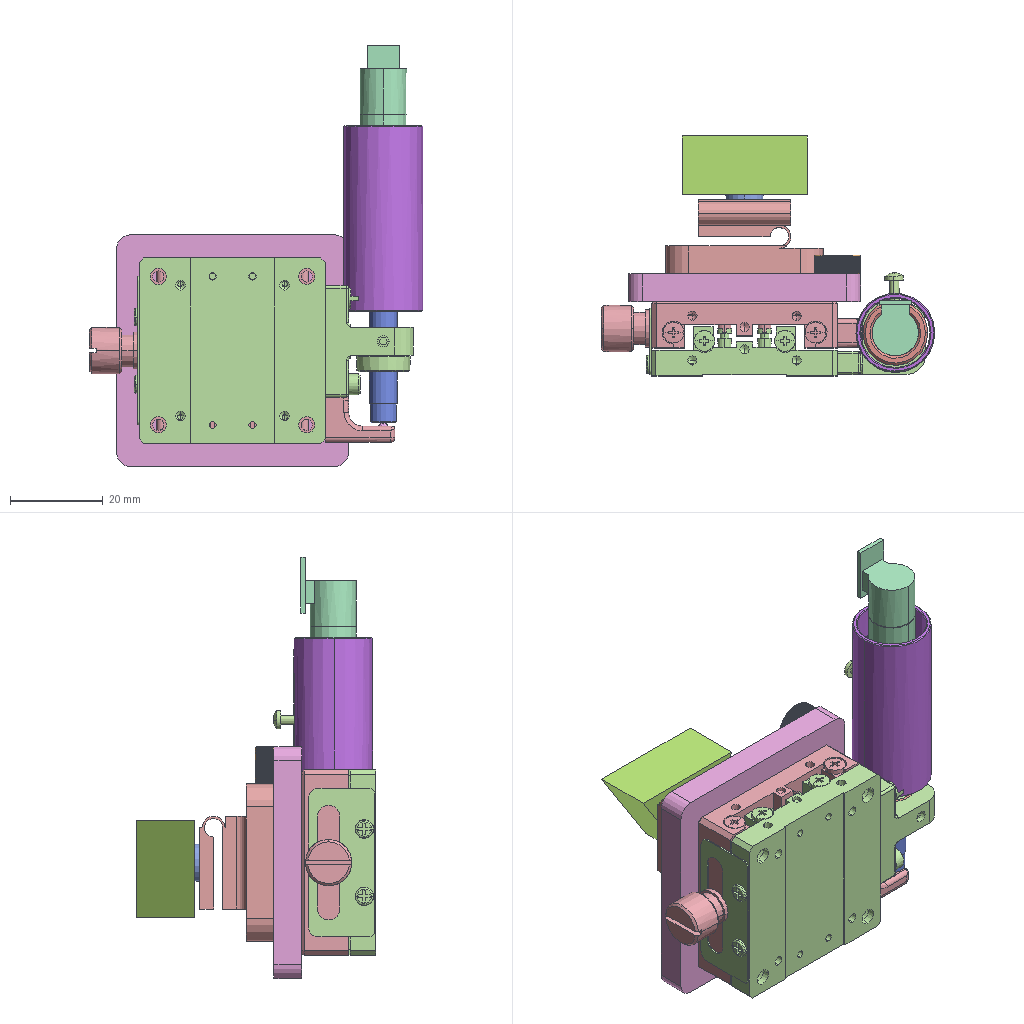Assembly | SolidWorks | 18 different items | 18 placed | box 72 x 52 x 91 mm
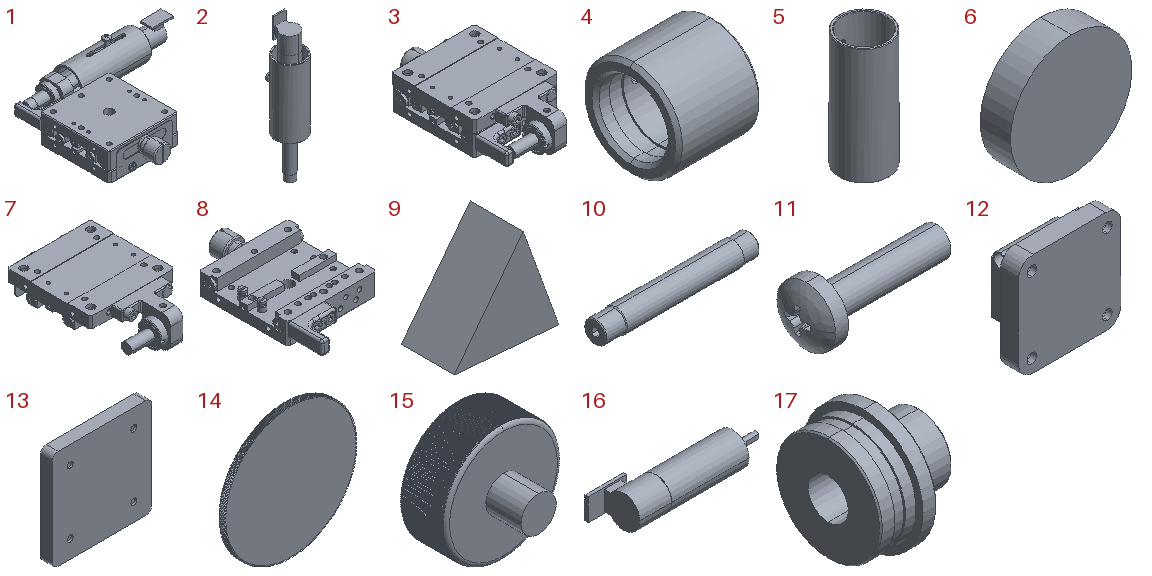Parts list (item | name | quantity | parent item | size | volume | features):
1 | (subassembly) | x1 | - | 85.8 x 71.9 x 22.138 mm | 31070 mm3 | -
2 | (subassembly) | x1 | in 1 | 17 x 21.434 x 81.3 mm | 6886 mm3 | -
3 | (subassembly) | x1 | in 1 | 40 x 69.9 x 16 mm | 24184 mm3 | -
4 | - | x1 | in 2 | 12 x 14 x 14 mm | 997.34 mm3 | features BaseBody 1
5 | - | x1 | in 2 | 17 x 17 x 40 mm | 1956 mm3 | features BaseBody 1, MoveFace 1
6 | - | x1 | - | 8 x 2 x 8 mm | 100.531 mm3 | features Extrusion 1
7 | - | x1 | in 3 | 40 x 60.2 x 15.5 mm | 12589 mm3 | features BaseBody 14
8 | - | x1 | in 3 | 40 x 65.9 x 10.8 mm | 11595 mm3 | features BaseBody 12
9 | - | x1 | - | 24.913 x 12.7 x 23.516 mm | 3608 mm3 | features Extrusion 1
10 | - | x1 | in 2 | 39 x 6 x 6 mm | 1057 mm3 | features BaseBody 1
11 | - | x1 | in 2 | 9.576 x 4 x 4 mm | 40.085 mm3 | features BaseBody 1
12 | - | x1 | - | 34 x 16 x 34 mm | 8130 mm3 | features ICE 9, Extrusion 1, Fillet 1
13 | - | x1 | - | 50 x 6 x 50 mm | 9918 mm3 | features ICE 4, Extrusion 1, Fillet 1
14 | - | x1 | - | 45.5 x 2 x 45.5 mm | 3201 mm3 | features CirPattern 3, ICE 3, Extrusion 1
15 | - | x1 | - | 10 x 7 x 10 mm | 331.248 mm3 | features ICE 2, CirPattern 1, Extrusion 1, Fillet 1
16 | - | x1 | in 2 | 46.3 x 12 x 10 mm | 2836 mm3 | features BaseBody 1
17 | - | x1 | - | 13 x 17 x 17 mm | 1399 mm3 | features BaseBody 1
18 | Lead Screw Nut-EC-OS1P1D-CUNO-0804A | x1 | - | - | - | -
Mates (type | each side: item.copy, entity, surface, feature):
In the top assembly
Coincident | 12.1 face plane Cut-Extrude8 | 6.1 face plane Boss-Extrude1
Concentric | 12.1 edge | 6.1 face cylinder Boss-Extrude1
Coincident | 6.1 face plane Boss-Extrude1 | 9.1 face plane Boss-Extrude1
Parallel | 12.1 face plane Boss-Extrude1 | 9.1 face plane Boss-Extrude1
Coincident | 13.1 face plane Boss-Extrude1 | 14.1 face plane Boss-Extrude1
Concentric | 13.1 face cylinder Cut-Extrude2 | 15.1 face cylinder Boss-Extrude1
Coincident | 13.1 face plane Boss-Extrude1 | 15.1 face plane Boss-Extrude2
Coincident | 12.1 face plane Boss-Extrude1 | 14.1 face plane Boss-Extrude1
DistanceDim | 12.1 face plane Boss-Extrude1 | 13.1 face plane Boss-Extrude1 | 2 times
Concentric | 13.1 face cylinder Cut-Extrude4 | 8.1 face cylinder Input 2
Concentric | 13.1 face cylinder Cut-Extrude4 | 8.1 edge
Coincident | 13.1 face plane Cut-Extrude3 | 8.1 face plane Input 2
In subassembly 1
Concentric | 7.1 face cylinder Input 10 | 10.1 face cylinder Input 1
Coincident | 7.1 face plane Input 10 | 10.1 face plane Input 1
Parallel | 8.2 face plane Input 2 | 16.1 face plane Input 1
In subassembly 2
Concentric | 16.2 face cylinder Input 1 | 10.2 face cylinder Input 1
Concentric | 16.2 face cylinder Input 1 | 4.1 face cylinder Input 1
Coincident | 16.2 face plane Input 1 | 4.1 face plane Input 1
Concentric | 4.1 face cylinder Input 1 | 11.1 face cylinder Input 1
Coincident | 16.2 face plane Input 1 | 10.2 face plane Input 1 | 2 times